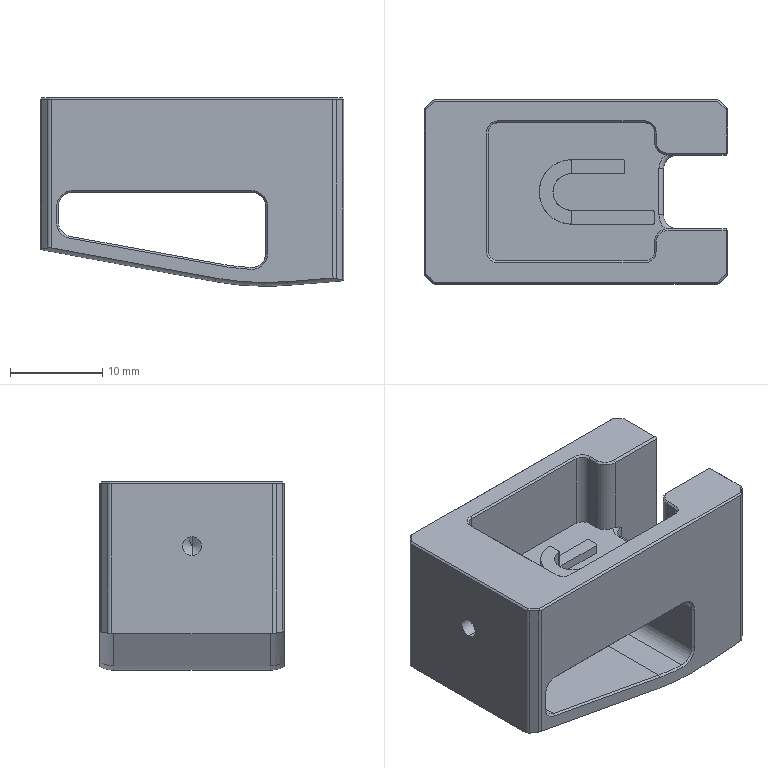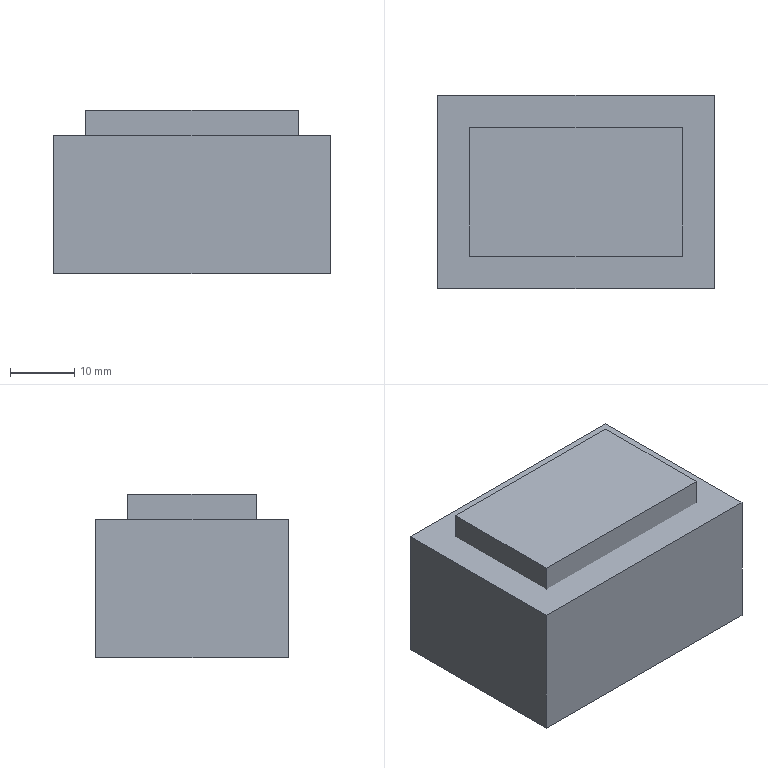CAM job | NX | 3+2 milling | part box 33 x 20 x 20.478 mm | stock box 43 x 30 x 25.478 mm
Tools:
number,name,description,diameter,corner_radius,flute_length,length,flutes
19,D80,Milling Tool-5 Parameters,80.0,0.0,50.0,75.0,2
15,D10,Milling Tool-5 Parameters,10.0,0.0,50.0,75.0,2
12,D6,Milling Tool-5 Parameters,6.0,0.0,50.0,75.0,2
16,D3,Milling Tool-5 Parameters,3.0,0.0,50.0,75.0,2
11,D4,Milling Tool-5 Parameters,4.0,0.0,50.0,75.0,2
17,D2,Milling Tool-5 Parameters,2.0,0.0,50.0,75.0,2
18,D1,Milling Tool-5 Parameters,1.0,0.0,50.0,75.0,2
24,D2R0.5,Milling Tool-5 Parameters,2.0,0.5,50.0,75.0,2
1,D6A45,Milling Tool-5 Parameters,6.0,0.0,50.0,75.0,2
Operations:
program,operation,operation_type,tool,method,geometry_group,spindle_rpm,surface_speed,feed_per_tooth,feed_cut,feed_plunge,cut_length_mm,path_length_mm,cut_time_min,machine_time_min
1,FLOOR_WALL,VolumeBased25DMillingOperation,D80,METHOD,A,6500.0,1633.0,0.1154,1500.0,100.0,135.0,155.0,0.09,0.092
1,ADAPTIVE_MILLING,CavityMilling,D10,METHOD,A,9500.0,298.0,0.1579,3000.0,1000.0,1068.501,1125.458,0.3582,0.3639
1,ZLEVEL_PROFILE,ZLevelMilling,D6,METHOD,A,9500.0,179.0,0.0947,1800.0,100.0,745.6,956.328,0.4142,0.4353
1,CAVITY_MILL,CavityMilling,D6,METHOD,A,9500.0,179.0,0.1316,2500.0,1000.0,1623.89,1854.567,0.9749,0.998
1,CAVITY_MILL_COPY,CavityMilling,D4,METHOD,A,9500.0,119.0,0.0947,1800.0,1000.0,1784.637,2730.084,1.204,1.298
1,FLOOR_WALL_1,VolumeBased25DMillingOperation,D4,METHOD,A,9500.0,119.0,0.0658,1250.0,100.0,419.416,839.501,0.3355,0.3775
1,ZLEVEL_PROFILE_COPY,ZLevelMilling,D3,METHOD,A,9500.0,89.0,0.0526,1000.0,100.0,1271.245,1914.952,1.271,1.336
1,CAVITY_MILL_COPY_COPY,CavityMilling,D2,METHOD,A,9500.0,59.0,0.0526,1000.0,1000.0,2457.475,4004.249,2.458,2.612
1,FLOOR_WALL_1_COPY,VolumeBased25DMillingOperation,D2,METHOD,A,9500.0,59.0,0.0526,1000.0,100.0,562.578,897.563,0.5626,0.5961
1,CAVITY_MILL_COPY_COPY_COPY,CavityMilling,D1,METHOD,A,9500.0,29.0,0.0447,850.0,1000.0,122.13,172.806,0.14,0.145
1,ZLEVEL_PROFILE_1,ZLevelMilling,D2R0.5,METHOD,A,9500.0,119.0,0.1316,2500.0,100.0,100.565,138.181,0.0402,0.044
1,PLANAR_MILL_COPY_COPY_COPY_COPY_COPY_COPY_1,PlanarMilling,D6A45,METHOD,A,9500.0,179.0,0.0658,1250.0,100.0,179.159,199.159,0.1433,0.1453
1,刀补,ZLevelMilling,D6,METHOD,A,9500.0,179.0,0.0632,1200.0,100.0,413.822,514.404,0.3449,0.3549
2,CAVITY_MILL_1,CavityMilling,D80,METHOD,B,6500.0,1633.0,0.1154,1500.0,100.0,1711.636,2094.157,1.141,1.179
2,FIXED_CONTOUR,SurfaceContour,D6,METHOD,B,9500.0,0.0,0.0,2500.0,1000.0,2046.409,2099.209,0.8221,0.8274
2,FIXED_CONTOUR_COPY,SurfaceContour,D2R0.5,METHOD,B,9500.0,0.0,0.0,2500.0,1000.0,7036.913,7091.314,2.817,2.823
3,PLANAR_MILL,PlanarMilling,D4,METHOD,C,9500.0,119.0,0.1158,2200.0,1000.0,5482.638,5815.485,3.814,3.847
3,PLANAR_MILL_COPY,PlanarMilling,D4,METHOD,C,9500.0,119.0,0.0632,1200.0,1000.0,183.419,281.493,0.154,0.1638
3,PLANAR_MILL_COPY_1,PlanarMilling,D3,METHOD,C,9500.0,89.0,0.0526,1000.0,1000.0,1624.57,2406.53,1.625,1.703
3,PLANAR_MILL_COPY_COPY_COPY_COPY_COPY_COPY_1_COPY,PlanarMilling,D6A45,METHOD,C,9500.0,179.0,0.0658,1250.0,100.0,55.705,114.705,0.0446,0.0505